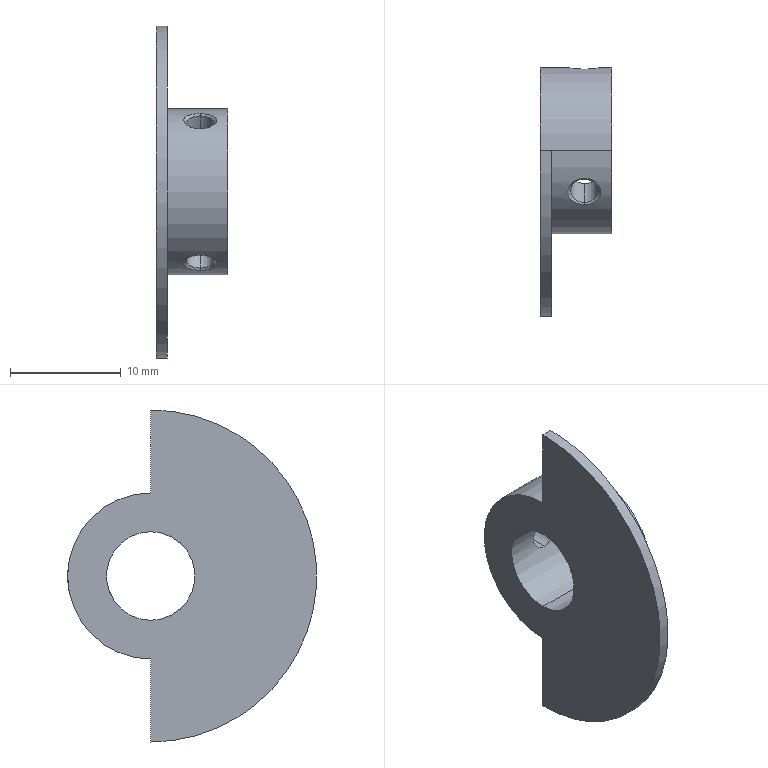Part | SolidWorks | features BaseBody 1 | 1 solid | 22 faces | box 6.5 x 22.5 x 30 mm | volume 1036 mm3 | cylinder 11 | cone 6 | plane 5 | commonest cylinder face diameters 2.459 x6 8 x2 15 x2 30 x1
STEP:
#1=CARTESIAN_POINT('',(4.,7.373,1.373));
#2=VERTEX_POINT('',#1);
#3=CARTESIAN_POINT('',(4.,7.373,-1.373));
#4=VERTEX_POINT('',#3);
#5=CARTESIAN_POINT('',(4.,7.373,1.373));
#6=CARTESIAN_POINT('',(3.812,7.373,1.373));
#7=CARTESIAN_POINT('',(3.623,7.38,1.34));
#8=CARTESIAN_POINT('',(3.27,7.402,1.211));
#9=CARTESIAN_POINT('',(3.105,7.418,1.115));
#10=CARTESIAN_POINT('',(2.821,7.451,0.8664));
#11=CARTESIAN_POINT('',(2.704,7.468,0.7143));
#12=CARTESIAN_POINT('',(2.543,7.493,0.3737));
#13=CARTESIAN_POINT('',(2.5,7.5,0.1847));
#14=CARTESIAN_POINT('',(2.5,7.5,-0.09668));
#15=CARTESIAN_POINT('',(2.511,7.498,-0.1919));
#16=CARTESIAN_POINT('',(2.554,7.491,-0.3755));
#17=CARTESIAN_POINT('',(2.585,7.486,-0.4636));
#18=CARTESIAN_POINT('',(2.666,7.474,-0.6329));
#19=CARTESIAN_POINT('',(2.716,7.466,-0.7143));
#20=CARTESIAN_POINT('',(2.83,7.451,-0.8624));
#21=CARTESIAN_POINT('',(2.894,7.442,-0.9303));
#22=CARTESIAN_POINT('',(3.035,7.426,-1.054));
#23=CARTESIAN_POINT('',(3.113,7.418,-1.109));
#24=CARTESIAN_POINT('',(3.274,7.403,-1.204));
#25=CARTESIAN_POINT('',(3.358,7.396,-1.244));
#26=CARTESIAN_POINT('',(3.624,7.379,-1.341));
#27=CARTESIAN_POINT('',(3.81,7.373,-1.373));
#28=CARTESIAN_POINT('',(4.,7.373,-1.373));
#29=B_SPLINE_CURVE_WITH_KNOTS('',3,(#5,#6,#7,#8,#9,#10,#11,#12,#13,#14,#15,#16,#17,#18,#19,#20,#21,#22,#23,#24,#25,#26,#27,#28),.UNSPECIFIED.,.F.,.F.,(4,2,2,2,2,2,2,2,2,2,2,4),(0.0008214,0.001385,0.001948,0.002512,0.003075,0.003357,0.003639,0.003921,0.004202,0.004484,0.004766,0.005329),.UNSPECIFIED.);
#30=EDGE_CURVE('',#2,#4,#29,.T.);
#31=ORIENTED_EDGE('',*,*,#30,.T.);
#32=CARTESIAN_POINT('',(4.,7.373,-1.373));
#33=CARTESIAN_POINT('',(4.19,7.373,-1.373));
#34=CARTESIAN_POINT('',(4.376,7.379,-1.341));
#35=CARTESIAN_POINT('',(4.731,7.402,-1.211));
#36=CARTESIAN_POINT('',(4.896,7.418,-1.115));
#37=CARTESIAN_POINT('',(5.178,7.451,-0.8673));
#38=CARTESIAN_POINT('',(5.295,7.468,-0.7151));
#39=CARTESIAN_POINT('',(5.416,7.486,-0.461));
#40=CARTESIAN_POINT('',(5.448,7.491,-0.3707));
#41=CARTESIAN_POINT('',(5.489,7.498,-0.1871));
#42=CARTESIAN_POINT('',(5.5,7.5,-0.09388));
#43=CARTESIAN_POINT('',(5.5,7.5,0.19));
#44=CARTESIAN_POINT('',(5.456,7.492,0.3767));
#45=CARTESIAN_POINT('',(5.335,7.474,0.6321));
#46=CARTESIAN_POINT('',(5.286,7.467,0.7115));
#47=CARTESIAN_POINT('',(5.172,7.451,0.8598));
#48=CARTESIAN_POINT('',(5.107,7.442,0.9292));
#49=CARTESIAN_POINT('',(4.895,7.418,1.115));
#50=CARTESIAN_POINT('',(4.73,7.402,1.212));
#51=CARTESIAN_POINT('',(4.377,7.38,1.34));
#52=CARTESIAN_POINT('',(4.188,7.373,1.373));
#53=CARTESIAN_POINT('',(4.,7.373,1.373));
#54=B_SPLINE_CURVE_WITH_KNOTS('',3,(#32,#33,#34,#35,#36,#37,#38,#39,#40,#41,#42,#43,#44,#45,#46,#47,#48,#49,#50,#51,#52,#53),.UNSPECIFIED.,.F.,.F.,(4,2,2,2,2,2,2,2,2,2,4),(0.005329,0.005893,0.006456,0.00702,0.007301,0.007583,0.008146,0.008428,0.00871,0.009273,0.009837),.UNSPECIFIED.);
#55=EDGE_CURVE('',#4,#2,#54,.T.);
#56=ORIENTED_EDGE('',*,*,#55,.T.);
#57=EDGE_LOOP('',(#31,#56));
#58=FACE_BOUND('',#57,.T.);
#59=CARTESIAN_POINT('',(1.,0.,7.5));
#60=VERTEX_POINT('',#59);
#61=CARTESIAN_POINT('',(0.,0.,7.5));
#62=VERTEX_POINT('',#61);
#63=CARTESIAN_POINT('',(1.,0.,7.5));
#64=DIRECTION('',(-1.,0.,0.));
#65=VECTOR('',#64,1000.);
#66=LINE('',#63,#65);
#67=EDGE_CURVE('',#60,#62,#66,.T.);
#68=ORIENTED_EDGE('',*,*,#67,.F.);
#69=CARTESIAN_POINT('',(6.5,0.,7.5));
#70=VERTEX_POINT('',#69);
#71=CARTESIAN_POINT('',(0.,0.,7.5));
#72=DIRECTION('',(1.,0.,0.));
#73=VECTOR('',#72,1000.);
#74=LINE('',#71,#73);
#75=EDGE_CURVE('',#60,#70,#74,.T.);
#76=ORIENTED_EDGE('',*,*,#75,.T.);
#77=CARTESIAN_POINT('',(6.5,0.,-7.5));
#78=VERTEX_POINT('',#77);
#79=CARTESIAN_POINT('',(6.5,0.,0.));
#80=DIRECTION('',(-1.,0.,0.));
#81=DIRECTION('',(0.,0.,-1.));
#82=AXIS2_PLACEMENT_3D('',#79,#80,#81);
#83=CIRCLE('',#82,7.5);
#84=EDGE_CURVE('',#70,#78,#83,.T.);
#85=ORIENTED_EDGE('',*,*,#84,.T.);
#86=CARTESIAN_POINT('',(1.,0.,-7.5));
#87=VERTEX_POINT('',#86);
#88=CARTESIAN_POINT('',(0.,0.,-7.5));
#89=DIRECTION('',(1.,0.,0.));
#90=VECTOR('',#89,1000.);
#91=LINE('',#88,#90);
#92=EDGE_CURVE('',#87,#78,#91,.T.);
#93=ORIENTED_EDGE('',*,*,#92,.F.);
#94=CARTESIAN_POINT('',(0.,0.,-7.5));
#95=VERTEX_POINT('',#94);
#96=CARTESIAN_POINT('',(0.,0.,-7.5));
#97=DIRECTION('',(-1.,0.,0.));
#98=VECTOR('',#97,1000.);
#99=LINE('',#96,#98);
#100=EDGE_CURVE('',#87,#95,#99,.T.);
#101=ORIENTED_EDGE('',*,*,#100,.T.);
#102=CARTESIAN_POINT('',(0.,0.,0.));
#103=DIRECTION('',(1.,0.,0.));
#104=DIRECTION('',(0.,0.,-1.));
#105=AXIS2_PLACEMENT_3D('',#102,#103,#104);
#106=CIRCLE('',#105,7.5);
#107=EDGE_CURVE('',#95,#62,#106,.T.);
#108=ORIENTED_EDGE('',*,*,#107,.T.);
#109=EDGE_LOOP('',(#68,#76,#85,#93,#101,#108));
#110=FACE_OUTER_BOUND('',#109,.T.);
#111=CARTESIAN_POINT('',(0.,0.,0.));
#112=DIRECTION('',(1.,0.,0.));
#113=DIRECTION('',(0.,0.,-1.));
#114=AXIS2_PLACEMENT_3D('',#111,#112,#113);
#115=CYLINDRICAL_SURFACE('',#114,7.5);
#116=ADVANCED_FACE('',(#58,#110),#115,.T.);
#117=CARTESIAN_POINT('',(4.,-2.968,2.682));
#118=VERTEX_POINT('',#117);
#119=CARTESIAN_POINT('',(4.,-0.8384,3.911));
#120=VERTEX_POINT('',#119);
#121=CARTESIAN_POINT('',(4.,-2.968,2.682));
#122=CARTESIAN_POINT('',(3.919,-2.968,2.682));
#123=CARTESIAN_POINT('',(3.837,-2.962,2.688));
#124=CARTESIAN_POINT('',(3.679,-2.94,2.713));
#125=CARTESIAN_POINT('',(3.602,-2.923,2.731));
#126=CARTESIAN_POINT('',(3.379,-2.856,2.801));
#127=CARTESIAN_POINT('',(3.245,-2.791,2.868));
#128=CARTESIAN_POINT('',(3.017,-2.619,3.025));
#129=CARTESIAN_POINT('',(2.926,-2.515,3.114));
#130=CARTESIAN_POINT('',(2.803,-2.275,3.294));
#131=CARTESIAN_POINT('',(2.77,-2.139,3.384));
#132=CARTESIAN_POINT('',(2.771,-1.86,3.545));
#133=CARTESIAN_POINT('',(2.803,-1.714,3.617));
#134=CARTESIAN_POINT('',(2.926,-1.441,3.735));
#135=CARTESIAN_POINT('',(3.017,-1.31,3.781));
#136=CARTESIAN_POINT('',(3.243,-1.089,3.851));
#137=CARTESIAN_POINT('',(3.378,-0.998,3.874));
#138=CARTESIAN_POINT('',(3.677,-0.8717,3.904));
#139=CARTESIAN_POINT('',(3.838,-0.8384,3.911));
#140=CARTESIAN_POINT('',(4.,-0.8384,3.911));
#141=B_SPLINE_CURVE_WITH_KNOTS('',3,(#121,#122,#123,#124,#125,#126,#127,#128,#129,#130,#131,#132,#133,#134,#135,#136,#137,#138,#139,#140),.UNSPECIFIED.,.F.,.F.,(4,2,2,2,2,2,2,2,2,4),(0.0002413,0.0004837,0.0007262,0.001211,0.001696,0.002181,0.002665,0.00315,0.003635,0.00412),.UNSPECIFIED.);
#142=EDGE_CURVE('',#118,#120,#141,.T.);
#143=ORIENTED_EDGE('',*,*,#142,.F.);
#144=CARTESIAN_POINT('',(4.,-0.8384,3.911));
#145=CARTESIAN_POINT('',(4.081,-0.8384,3.911));
#146=CARTESIAN_POINT('',(4.161,-0.8466,3.909));
#147=CARTESIAN_POINT('',(4.319,-0.8789,3.902));
#148=CARTESIAN_POINT('',(4.398,-0.9034,3.897));
#149=CARTESIAN_POINT('',(4.62,-0.9969,3.874));
#150=CARTESIAN_POINT('',(4.756,-1.089,3.851));
#151=CARTESIAN_POINT('',(4.982,-1.309,3.782));
#152=CARTESIAN_POINT('',(5.073,-1.439,3.735));
#153=CARTESIAN_POINT('',(5.166,-1.645,3.647));
#154=CARTESIAN_POINT('',(5.19,-1.717,3.614));
#155=CARTESIAN_POINT('',(5.221,-1.858,3.543));
#156=CARTESIAN_POINT('',(5.229,-1.929,3.505));
#157=CARTESIAN_POINT('',(5.23,-2.141,3.383));
#158=CARTESIAN_POINT('',(5.197,-2.274,3.294));
#159=CARTESIAN_POINT('',(5.073,-2.515,3.114));
#160=CARTESIAN_POINT('',(4.982,-2.62,3.025));
#161=CARTESIAN_POINT('',(4.756,-2.79,2.868));
#162=CARTESIAN_POINT('',(4.62,-2.857,2.801));
#163=CARTESIAN_POINT('',(4.324,-2.945,2.708));
#164=CARTESIAN_POINT('',(4.162,-2.968,2.682));
#165=CARTESIAN_POINT('',(4.,-2.968,2.682));
#166=B_SPLINE_CURVE_WITH_KNOTS('',3,(#144,#145,#146,#147,#148,#149,#150,#151,#152,#153,#154,#155,#156,#157,#158,#159,#160,#161,#162,#163,#164,#165),.UNSPECIFIED.,.F.,.F.,(4,2,2,2,2,2,2,2,2,2,4),(0.00412,0.004362,0.004605,0.00509,0.005575,0.005818,0.00606,0.006545,0.00703,0.007515,0.008),.UNSPECIFIED.);
#167=EDGE_CURVE('',#120,#118,#166,.T.);
#168=ORIENTED_EDGE('',*,*,#167,.F.);
#169=EDGE_LOOP('',(#143,#168));
#170=FACE_BOUND('',#169,.T.);
#171=CARTESIAN_POINT('',(4.,-0.8384,-3.911));
#172=VERTEX_POINT('',#171);
#173=CARTESIAN_POINT('',(4.,-2.968,-2.682));
#174=VERTEX_POINT('',#173);
#175=CARTESIAN_POINT('',(4.,-0.8384,-3.911));
#176=CARTESIAN_POINT('',(3.919,-0.8384,-3.911));
#177=CARTESIAN_POINT('',(3.837,-0.8468,-3.909));
#178=CARTESIAN_POINT('',(3.679,-0.8793,-3.902));
#179=CARTESIAN_POINT('',(3.602,-0.9032,-3.897));
#180=CARTESIAN_POINT('',(3.379,-0.9973,-3.874));
#181=CARTESIAN_POINT('',(3.245,-1.088,-3.851));
#182=CARTESIAN_POINT('',(3.017,-1.311,-3.781));
#183=CARTESIAN_POINT('',(2.926,-1.44,-3.735));
#184=CARTESIAN_POINT('',(2.803,-1.715,-3.617));
#185=CARTESIAN_POINT('',(2.77,-1.861,-3.545));
#186=CARTESIAN_POINT('',(2.771,-2.14,-3.383));
#187=CARTESIAN_POINT('',(2.803,-2.275,-3.293));
#188=CARTESIAN_POINT('',(2.926,-2.514,-3.115));
#189=CARTESIAN_POINT('',(3.017,-2.619,-3.025));
#190=CARTESIAN_POINT('',(3.243,-2.79,-2.869));
#191=CARTESIAN_POINT('',(3.378,-2.856,-2.801));
#192=CARTESIAN_POINT('',(3.677,-2.945,-2.707));
#193=CARTESIAN_POINT('',(3.838,-2.968,-2.682));
#194=CARTESIAN_POINT('',(4.,-2.968,-2.682));
#195=B_SPLINE_CURVE_WITH_KNOTS('',3,(#175,#176,#177,#178,#179,#180,#181,#182,#183,#184,#185,#186,#187,#188,#189,#190,#191,#192,#193,#194),.UNSPECIFIED.,.F.,.F.,(4,2,2,2,2,2,2,2,2,4),(0.0002413,0.0004837,0.0007262,0.001211,0.001696,0.002181,0.002665,0.00315,0.003635,0.00412),.UNSPECIFIED.);
#196=EDGE_CURVE('',#172,#174,#195,.T.);
#197=ORIENTED_EDGE('',*,*,#196,.F.);
#198=CARTESIAN_POINT('',(4.,-2.968,-2.682));
#199=CARTESIAN_POINT('',(4.081,-2.968,-2.682));
#200=CARTESIAN_POINT('',(4.161,-2.962,-2.688));
#201=CARTESIAN_POINT('',(4.319,-2.94,-2.712));
#202=CARTESIAN_POINT('',(4.398,-2.923,-2.731));
#203=CARTESIAN_POINT('',(4.62,-2.857,-2.801));
#204=CARTESIAN_POINT('',(4.756,-2.79,-2.868));
#205=CARTESIAN_POINT('',(4.982,-2.621,-3.024));
#206=CARTESIAN_POINT('',(5.073,-2.515,-3.114));
#207=CARTESIAN_POINT('',(5.166,-2.336,-3.248));
#208=CARTESIAN_POINT('',(5.19,-2.271,-3.294));
#209=CARTESIAN_POINT('',(5.221,-2.139,-3.381));
#210=CARTESIAN_POINT('',(5.229,-2.071,-3.423));
#211=CARTESIAN_POINT('',(5.23,-1.859,-3.545));
#212=CARTESIAN_POINT('',(5.197,-1.715,-3.617));
#213=CARTESIAN_POINT('',(5.073,-1.439,-3.735));
#214=CARTESIAN_POINT('',(4.982,-1.31,-3.781));
#215=CARTESIAN_POINT('',(4.756,-1.089,-3.851));
#216=CARTESIAN_POINT('',(4.62,-0.9971,-3.874));
#217=CARTESIAN_POINT('',(4.324,-0.8723,-3.904));
#218=CARTESIAN_POINT('',(4.162,-0.8384,-3.911));
#219=CARTESIAN_POINT('',(4.,-0.8384,-3.911));
#220=B_SPLINE_CURVE_WITH_KNOTS('',3,(#198,#199,#200,#201,#202,#203,#204,#205,#206,#207,#208,#209,#210,#211,#212,#213,#214,#215,#216,#217,#218,#219),.UNSPECIFIED.,.F.,.F.,(4,2,2,2,2,2,2,2,2,2,4),(0.00412,0.004362,0.004605,0.00509,0.005575,0.005818,0.00606,0.006545,0.00703,0.007515,0.008),.UNSPECIFIED.);
#221=EDGE_CURVE('',#174,#172,#220,.T.);
#222=ORIENTED_EDGE('',*,*,#221,.F.);
#223=EDGE_LOOP('',(#197,#222));
#224=FACE_BOUND('',#223,.T.);
#225=CARTESIAN_POINT('',(0.,0.,-4.));
#226=VERTEX_POINT('',#225);
#227=CARTESIAN_POINT('',(0.,0.,4.));
#228=VERTEX_POINT('',#227);
#229=CARTESIAN_POINT('',(0.,0.,0.));
#230=DIRECTION('',(-1.,0.,0.));
#231=DIRECTION('',(0.,0.,-1.));
#232=AXIS2_PLACEMENT_3D('',#229,#230,#231);
#233=CIRCLE('',#232,4.);
#234=EDGE_CURVE('',#226,#228,#233,.T.);
#235=ORIENTED_EDGE('',*,*,#234,.T.);
#236=CARTESIAN_POINT('',(6.5,0.,4.));
#237=VERTEX_POINT('',#236);
#238=CARTESIAN_POINT('',(6.5,0.,4.));
#239=DIRECTION('',(1.,0.,0.));
#240=VECTOR('',#239,1000.);
#241=LINE('',#238,#240);
#242=EDGE_CURVE('',#228,#237,#241,.T.);
#243=ORIENTED_EDGE('',*,*,#242,.T.);
#244=CARTESIAN_POINT('',(6.5,0.,-4.));
#245=VERTEX_POINT('',#244);
#246=CARTESIAN_POINT('',(6.5,0.,0.));
#247=DIRECTION('',(-1.,0.,0.));
#248=DIRECTION('',(0.,0.,-1.));
#249=AXIS2_PLACEMENT_3D('',#246,#247,#248);
#250=CIRCLE('',#249,4.);
#251=EDGE_CURVE('',#245,#237,#250,.T.);
#252=ORIENTED_EDGE('',*,*,#251,.F.);
#253=CARTESIAN_POINT('',(6.5,0.,-4.));
#254=DIRECTION('',(1.,0.,0.));
#255=VECTOR('',#254,1000.);
#256=LINE('',#253,#255);
#257=EDGE_CURVE('',#226,#245,#256,.T.);
#258=ORIENTED_EDGE('',*,*,#257,.F.);
#259=EDGE_LOOP('',(#235,#243,#252,#258));
#260=FACE_OUTER_BOUND('',#259,.T.);
#261=CARTESIAN_POINT('',(6.5,0.,0.));
#262=DIRECTION('',(1.,0.,0.));
#263=DIRECTION('',(0.,0.,-1.));
#264=AXIS2_PLACEMENT_3D('',#261,#262,#263);
#265=CYLINDRICAL_SURFACE('',#264,4.);
#266=ADVANCED_FACE('',(#170,#224,#260),#265,.F.);
#267=CARTESIAN_POINT('',(4.,-4.68,-5.646));
#268=VERTEX_POINT('',#267);
#269=CARTESIAN_POINT('',(4.,-2.55,-6.876));
#270=VERTEX_POINT('',#269);
#271=CARTESIAN_POINT('',(4.,-3.615,-6.261));
#272=DIRECTION('',(0.,-0.5,-0.866));
#273=DIRECTION('',(0.,0.866,-0.5));
#274=AXIS2_PLACEMENT_3D('',#271,#272,#273);
#275=CIRCLE('',#274,1.229);
#276=EDGE_CURVE('',#268,#270,#275,.T.);
#277=ORIENTED_EDGE('',*,*,#276,.F.);
#278=CARTESIAN_POINT('',(4.,-4.876,-5.699));
#279=VERTEX_POINT('',#278);
#280=CARTESIAN_POINT('',(4.,-5.053,-5.746));
#281=DIRECTION('',(0.,-0.9659,-0.2588));
#282=VECTOR('',#281,1000.);
#283=LINE('',#280,#282);
#284=EDGE_CURVE('',#268,#279,#283,.T.);
#285=ORIENTED_EDGE('',*,*,#284,.T.);
#286=CARTESIAN_POINT('',(4.,-2.497,-7.072));
#287=VERTEX_POINT('',#286);
#288=CARTESIAN_POINT('',(4.,-2.497,-7.072));
#289=CARTESIAN_POINT('',(3.812,-2.497,-7.072));
#290=CARTESIAN_POINT('',(3.623,-2.529,-7.061));
#291=CARTESIAN_POINT('',(3.27,-2.652,-7.016));
#292=CARTESIAN_POINT('',(3.105,-2.743,-6.982));
#293=CARTESIAN_POINT('',(2.821,-2.975,-6.886));
#294=CARTESIAN_POINT('',(2.704,-3.115,-6.825));
#295=CARTESIAN_POINT('',(2.543,-3.423,-6.676));
#296=CARTESIAN_POINT('',(2.5,-3.59,-6.588));
#297=CARTESIAN_POINT('',(2.5,-3.834,-6.447));
#298=CARTESIAN_POINT('',(2.511,-3.915,-6.398));
#299=CARTESIAN_POINT('',(2.554,-4.071,-6.3));
#300=CARTESIAN_POINT('',(2.585,-4.145,-6.251));
#301=CARTESIAN_POINT('',(2.666,-4.285,-6.156));
#302=CARTESIAN_POINT('',(2.716,-4.352,-6.109));
#303=CARTESIAN_POINT('',(2.83,-4.472,-6.021));
#304=CARTESIAN_POINT('',(2.894,-4.527,-5.98));
#305=CARTESIAN_POINT('',(3.035,-4.626,-5.904));
#306=CARTESIAN_POINT('',(3.113,-4.67,-5.869));
#307=CARTESIAN_POINT('',(3.274,-4.744,-5.809));
#308=CARTESIAN_POINT('',(3.358,-4.775,-5.784));
#309=CARTESIAN_POINT('',(3.624,-4.851,-5.721));
#310=CARTESIAN_POINT('',(3.811,-4.876,-5.699));
#311=CARTESIAN_POINT('',(4.,-4.876,-5.699));
#312=B_SPLINE_CURVE_WITH_KNOTS('',3,(#288,#289,#290,#291,#292,#293,#294,#295,#296,#297,#298,#299,#300,#301,#302,#303,#304,#305,#306,#307,#308,#309,#310,#311),.UNSPECIFIED.,.F.,.F.,(4,2,2,2,2,2,2,2,2,2,2,4),(0.001763,0.002329,0.002895,0.003461,0.004027,0.00431,0.004593,0.004876,0.005159,0.005442,0.005725,0.006291),.UNSPECIFIED.);
#313=EDGE_CURVE('',#287,#279,#312,.T.);
#314=ORIENTED_EDGE('',*,*,#313,.F.);
#315=CARTESIAN_POINT('',(4.,-2.45,-7.249));
#316=DIRECTION('',(0.,0.2588,-0.9659));
#317=VECTOR('',#316,1000.);
#318=LINE('',#315,#317);
#319=EDGE_CURVE('',#270,#287,#318,.T.);
#320=ORIENTED_EDGE('',*,*,#319,.F.);
#321=EDGE_LOOP('',(#277,#285,#314,#320));
#322=FACE_OUTER_BOUND('',#321,.T.);
#323=CARTESIAN_POINT('',(4.,-3.751,-6.498));
#324=DIRECTION('',(0.,-0.5,-0.866));
#325=DIRECTION('',(0.,0.866,-0.5));
#326=AXIS2_PLACEMENT_3D('',#323,#324,#325);
#327=CONICAL_SURFACE('',#326,1.503,0.7854);
#328=ADVANCED_FACE('',(#322),#327,.F.);
#329=CARTESIAN_POINT('',(4.,7.229,-1.23));
#330=VERTEX_POINT('',#329);
#331=CARTESIAN_POINT('',(4.,7.229,1.23));
#332=VERTEX_POINT('',#331);
#333=CARTESIAN_POINT('',(4.,7.229,0.));
#334=DIRECTION('',(0.,1.,0.));
#335=DIRECTION('',(0.,0.,1.));
#336=AXIS2_PLACEMENT_3D('',#333,#334,#335);
#337=CIRCLE('',#336,1.23);
#338=EDGE_CURVE('',#330,#332,#337,.T.);
#339=ORIENTED_EDGE('',*,*,#338,.F.);
#340=CARTESIAN_POINT('',(4.,7.502,-1.502));
#341=DIRECTION('',(0.,0.7071,-0.7071));
#342=VECTOR('',#341,1000.);
#343=LINE('',#340,#342);
#344=EDGE_CURVE('',#330,#4,#343,.T.);
#345=ORIENTED_EDGE('',*,*,#344,.T.);
#346=ORIENTED_EDGE('',*,*,#30,.F.);
#347=CARTESIAN_POINT('',(4.,7.502,1.502));
#348=DIRECTION('',(0.,0.7071,0.7071));
#349=VECTOR('',#348,1000.);
#350=LINE('',#347,#349);
#351=EDGE_CURVE('',#332,#2,#350,.T.);
#352=ORIENTED_EDGE('',*,*,#351,.F.);
#353=EDGE_LOOP('',(#339,#345,#346,#352));
#354=FACE_OUTER_BOUND('',#353,.T.);
#355=CARTESIAN_POINT('',(4.,7.502,0.));
#356=DIRECTION('',(0.,1.,0.));
#357=DIRECTION('',(0.,0.,1.));
#358=AXIS2_PLACEMENT_3D('',#355,#356,#357);
#359=CONICAL_SURFACE('',#358,1.502,0.7854);
#360=ADVANCED_FACE('',(#354),#359,.F.);
#361=CARTESIAN_POINT('',(4.,-2.55,6.876));
#362=VERTEX_POINT('',#361);
#363=CARTESIAN_POINT('',(4.,-4.68,5.646));
#364=VERTEX_POINT('',#363);
#365=CARTESIAN_POINT('',(4.,-3.615,6.261));
#366=DIRECTION('',(0.,-0.5,0.866));
#367=DIRECTION('',(0.,-0.866,-0.5));
#368=AXIS2_PLACEMENT_3D('',#365,#366,#367);
#369=CIRCLE('',#368,1.229);
#370=EDGE_CURVE('',#362,#364,#369,.T.);
#371=ORIENTED_EDGE('',*,*,#370,.F.);
#372=CARTESIAN_POINT('',(4.,-2.497,7.072));
#373=VERTEX_POINT('',#372);
#374=CARTESIAN_POINT('',(4.,-2.45,7.249));
#375=DIRECTION('',(0.,0.2588,0.9659));
#376=VECTOR('',#375,1000.);
#377=LINE('',#374,#376);
#378=EDGE_CURVE('',#362,#373,#377,.T.);
#379=ORIENTED_EDGE('',*,*,#378,.T.);
#380=CARTESIAN_POINT('',(4.,-4.876,5.699));
#381=VERTEX_POINT('',#380);
#382=CARTESIAN_POINT('',(4.,-4.876,5.699));
#383=CARTESIAN_POINT('',(3.812,-4.876,5.699));
#384=CARTESIAN_POINT('',(3.623,-4.85,5.721));
#385=CARTESIAN_POINT('',(3.27,-4.75,5.804));
#386=CARTESIAN_POINT('',(3.104,-4.674,5.867));
#387=CARTESIAN_POINT('',(2.822,-4.476,6.019));
#388=CARTESIAN_POINT('',(2.705,-4.354,6.109));
#389=CARTESIAN_POINT('',(2.583,-4.14,6.254));
#390=CARTESIAN_POINT('',(2.552,-4.066,6.303));
#391=CARTESIAN_POINT('',(2.51,-3.91,6.401));
#392=CARTESIAN_POINT('',(2.5,-3.829,6.45));
#393=CARTESIAN_POINT('',(2.5,-3.585,6.591));
#394=CARTESIAN_POINT('',(2.545,-3.417,6.679));
#395=CARTESIAN_POINT('',(2.666,-3.189,6.789));
#396=CARTESIAN_POINT('',(2.716,-3.115,6.823));
#397=CARTESIAN_POINT('',(2.83,-2.978,6.884));
#398=CARTESIAN_POINT('',(2.894,-2.915,6.911));
#399=CARTESIAN_POINT('',(3.035,-2.8,6.958));
#400=CARTESIAN_POINT('',(3.112,-2.748,6.979));
#401=CARTESIAN_POINT('',(3.274,-2.659,7.013));
#402=CARTESIAN_POINT('',(3.359,-2.621,7.027));
#403=CARTESIAN_POINT('',(3.535,-2.56,7.05));
#404=CARTESIAN_POINT('',(3.627,-2.536,7.058));
#405=CARTESIAN_POINT('',(3.813,-2.505,7.069));
#406=CARTESIAN_POINT('',(3.906,-2.497,7.072));
#407=CARTESIAN_POINT('',(4.,-2.497,7.072));
#408=B_SPLINE_CURVE_WITH_KNOTS('',3,(#382,#383,#384,#385,#386,#387,#388,#389,#390,#391,#392,#393,#394,#395,#396,#397,#398,#399,#400,#401,#402,#403,#404,#405,#406,#407),.UNSPECIFIED.,.F.,.F.,(4,2,2,2,2,2,2,2,2,2,2,2,4),(0.002987,0.003555,0.004124,0.004692,0.004976,0.005261,0.005829,0.006113,0.006398,0.006682,0.006966,0.00725,0.007535),.UNSPECIFIED.);
#409=EDGE_CURVE('',#381,#373,#408,.T.);
#410=ORIENTED_EDGE('',*,*,#409,.F.);
#411=CARTESIAN_POINT('',(4.,-5.053,5.746));
#412=DIRECTION('',(0.,-0.9659,0.2588));
#413=VECTOR('',#412,1000.);
#414=LINE('',#411,#413);
#415=EDGE_CURVE('',#364,#381,#414,.T.);
#416=ORIENTED_EDGE('',*,*,#415,.F.);
#417=EDGE_LOOP('',(#371,#379,#410,#416));
#418=FACE_OUTER_BOUND('',#417,.T.);
#419=CARTESIAN_POINT('',(4.,-3.751,6.498));
#420=DIRECTION('',(0.,-0.5,0.866));
#421=DIRECTION('',(0.,-0.866,-0.5));
#422=AXIS2_PLACEMENT_3D('',#419,#420,#421);
#423=CONICAL_SURFACE('',#422,1.503,0.7854);
#424=ADVANCED_FACE('',(#418),#423,.F.);
#425=ORIENTED_EDGE('',*,*,#196,.T.);
#426=CARTESIAN_POINT('',(4.,-2.565,-1.983));
#427=DIRECTION('',(0.,-0.5,-0.866));
#428=VECTOR('',#427,1000.);
#429=LINE('',#426,#428);
#430=EDGE_CURVE('',#174,#268,#429,.T.);
#431=ORIENTED_EDGE('',*,*,#430,.T.);
#432=ORIENTED_EDGE('',*,*,#276,.T.);
#433=CARTESIAN_POINT('',(4.,-0.4352,-3.213));
#434=DIRECTION('',(0.,-0.5,-0.866));
#435=VECTOR('',#434,1000.);
#436=LINE('',#433,#435);
#437=EDGE_CURVE('',#172,#270,#436,.T.);
#438=ORIENTED_EDGE('',*,*,#437,.F.);
#439=EDGE_LOOP('',(#425,#431,#432,#438));
#440=FACE_OUTER_BOUND('',#439,.T.);
#441=CARTESIAN_POINT('',(4.,-1.5,-2.598));
#442=DIRECTION('',(0.,-0.5,-0.866));
#443=DIRECTION('',(0.,0.866,-0.5));
#444=AXIS2_PLACEMENT_3D('',#441,#442,#443);
#445=CYLINDRICAL_SURFACE('',#444,1.23);
#446=ADVANCED_FACE('',(#440),#445,.F.);
#447=ORIENTED_EDGE('',*,*,#142,.T.);
#448=CARTESIAN_POINT('',(4.,-0.4352,3.213));
#449=DIRECTION('',(0.,-0.5,0.866));
#450=VECTOR('',#449,1000.);
#451=LINE('',#448,#450);
#452=EDGE_CURVE('',#120,#362,#451,.T.);
#453=ORIENTED_EDGE('',*,*,#452,.T.);
#454=ORIENTED_EDGE('',*,*,#370,.T.);
#455=CARTESIAN_POINT('',(4.,-2.565,1.983));
#456=DIRECTION('',(0.,-0.5,0.866));
#457=VECTOR('',#456,1000.);
#458=LINE('',#455,#457);
#459=EDGE_CURVE('',#118,#364,#458,.T.);
#460=ORIENTED_EDGE('',*,*,#459,.F.);
#461=EDGE_LOOP('',(#447,#453,#454,#460));
#462=FACE_OUTER_BOUND('',#461,.T.);
#463=CARTESIAN_POINT('',(4.,-1.5,2.598));
#464=DIRECTION('',(0.,-0.5,0.866));
#465=DIRECTION('',(0.,-0.866,-0.5));
#466=AXIS2_PLACEMENT_3D('',#463,#464,#465);
#467=CYLINDRICAL_SURFACE('',#466,1.23);
#468=ADVANCED_FACE('',(#462),#467,.F.);
#469=CARTESIAN_POINT('',(4.,3.806,1.23));
#470=VERTEX_POINT('',#469);
#471=CARTESIAN_POINT('',(4.,3.806,-1.23));
#472=VERTEX_POINT('',#471);
#473=CARTESIAN_POINT('',(4.,3.806,1.23));
#474=CARTESIAN_POINT('',(3.919,3.806,1.23));
#475=CARTESIAN_POINT('',(3.837,3.809,1.221));
#476=CARTESIAN_POINT('',(3.679,3.819,1.19));
#477=CARTESIAN_POINT('',(3.602,3.826,1.166));
#478=CARTESIAN_POINT('',(3.379,3.854,1.073));
#479=CARTESIAN_POINT('',(3.245,3.879,0.9834));
#480=CARTESIAN_POINT('',(3.017,3.93,0.7555));
#481=CARTESIAN_POINT('',(2.926,3.954,0.6205));
#482=CARTESIAN_POINT('',(2.803,3.99,0.3233));
#483=CARTESIAN_POINT('',(2.77,4.,0.1609));
#484=CARTESIAN_POINT('',(2.771,4.,-0.1613));
#485=CARTESIAN_POINT('',(2.803,3.99,-0.324));
#486=CARTESIAN_POINT('',(2.926,3.955,-0.6197));
#487=CARTESIAN_POINT('',(3.017,3.93,-0.7558));
#488=CARTESIAN_POINT('',(3.243,3.879,-0.9819));
#489=CARTESIAN_POINT('',(3.378,3.854,-1.073));
#490=CARTESIAN_POINT('',(3.677,3.817,-1.197));
#491=CARTESIAN_POINT('',(3.838,3.806,-1.23));
#492=CARTESIAN_POINT('',(4.,3.806,-1.23));
#493=B_SPLINE_CURVE_WITH_KNOTS('',3,(#473,#474,#475,#476,#477,#478,#479,#480,#481,#482,#483,#484,#485,#486,#487,#488,#489,#490,#491,#492),.UNSPECIFIED.,.F.,.F.,(4,2,2,2,2,2,2,2,2,4),(0.0002413,0.0004837,0.0007262,0.001211,0.001696,0.002181,0.002665,0.00315,0.003635,0.00412),.UNSPECIFIED.);
#494=EDGE_CURVE('',#470,#472,#493,.T.);
#495=ORIENTED_EDGE('',*,*,#494,.T.);
#496=CARTESIAN_POINT('',(4.,3.,-1.23));
#497=DIRECTION('',(0.,1.,0.));
#498=VECTOR('',#497,1000.);
#499=LINE('',#496,#498);
#500=EDGE_CURVE('',#472,#330,#499,.T.);
#501=ORIENTED_EDGE('',*,*,#500,.T.);
#502=ORIENTED_EDGE('',*,*,#338,.T.);
#503=CARTESIAN_POINT('',(4.,3.,1.23));
#504=DIRECTION('',(0.,1.,0.));
#505=VECTOR('',#504,1000.);
#506=LINE('',#503,#505);
#507=EDGE_CURVE('',#470,#332,#506,.T.);
#508=ORIENTED_EDGE('',*,*,#507,.F.);
#509=EDGE_LOOP('',(#495,#501,#502,#508));
#510=FACE_OUTER_BOUND('',#509,.T.);
#511=CARTESIAN_POINT('',(4.,3.,0.));
#512=DIRECTION('',(0.,1.,0.));
#513=DIRECTION('',(0.,0.,1.));
#514=AXIS2_PLACEMENT_3D('',#511,#512,#513);
#515=CYLINDRICAL_SURFACE('',#514,1.23);
#516=ADVANCED_FACE('',(#510),#515,.F.);
#517=ORIENTED_EDGE('',*,*,#107,.F.);
#518=CARTESIAN_POINT('',(0.,0.,-15.));
#519=VERTEX_POINT('',#518);
#520=CARTESIAN_POINT('',(0.,0.,0.));
#521=DIRECTION('',(0.,0.,1.));
#522=VECTOR('',#521,1000.);
#523=LINE('',#520,#522);
#524=EDGE_CURVE('',#519,#95,#523,.T.);
#525=ORIENTED_EDGE('',*,*,#524,.F.);
#526=CARTESIAN_POINT('',(0.,0.,15.));
#527=VERTEX_POINT('',#526);
#528=CARTESIAN_POINT('',(0.,0.,0.));
#529=DIRECTION('',(1.,0.,0.));
#530=DIRECTION('',(0.,0.,-1.));
#531=AXIS2_PLACEMENT_3D('',#528,#529,#530);
#532=CIRCLE('',#531,15.);
#533=EDGE_CURVE('',#527,#519,#532,.T.);
#534=ORIENTED_EDGE('',*,*,#533,.F.);
#535=CARTESIAN_POINT('',(0.,0.,0.));
#536=DIRECTION('',(0.,0.,1.));
#537=VECTOR('',#536,1000.);
#538=LINE('',#535,#537);
#539=EDGE_CURVE('',#62,#527,#538,.T.);
#540=ORIENTED_EDGE('',*,*,#539,.F.);
#541=EDGE_LOOP('',(#517,#525,#534,#540));
#542=FACE_OUTER_BOUND('',#541,.T.);
#543=ORIENTED_EDGE('',*,*,#234,.F.);
#544=CARTESIAN_POINT('',(0.,0.,0.));
#545=DIRECTION('',(-1.,0.,0.));
#546=DIRECTION('',(0.,0.,-1.));
#547=AXIS2_PLACEMENT_3D('',#544,#545,#546);
#548=CIRCLE('',#547,4.);
#549=EDGE_CURVE('',#228,#226,#548,.T.);
#550=ORIENTED_EDGE('',*,*,#549,.F.);
#551=EDGE_LOOP('',(#543,#550));
#552=FACE_BOUND('',#551,.T.);
#553=CARTESIAN_POINT('',(0.,-15.,0.));
#554=DIRECTION('',(1.,0.,0.));
#555=DIRECTION('',(0.,0.,-1.));
#556=AXIS2_PLACEMENT_3D('',#553,#554,#555);
#557=PLANE('',#556);
#558=ADVANCED_FACE('',(#542,#552),#557,.F.);
#559=CARTESIAN_POINT('',(1.,0.,15.));
#560=VERTEX_POINT('',#559);
#561=CARTESIAN_POINT('',(1.,0.,15.));
#562=DIRECTION('',(0.,0.,-1.));
#563=VECTOR('',#562,1000.);
#564=LINE('',#561,#563);
#565=EDGE_CURVE('',#560,#60,#564,.T.);
#566=ORIENTED_EDGE('',*,*,#565,.T.);
#567=ORIENTED_EDGE('',*,*,#67,.T.);
#568=ORIENTED_EDGE('',*,*,#539,.T.);
#569=CARTESIAN_POINT('',(1.,0.,15.));
#570=DIRECTION('',(1.,0.,0.));
#571=VECTOR('',#570,1000.);
#572=LINE('',#569,#571);
#573=EDGE_CURVE('',#527,#560,#572,.T.);
#574=ORIENTED_EDGE('',*,*,#573,.T.);
#575=EDGE_LOOP('',(#566,#567,#568,#574));
#576=FACE_OUTER_BOUND('',#575,.T.);
#577=CARTESIAN_POINT('',(1.,0.,15.));
#578=DIRECTION('',(0.,1.,0.));
#579=DIRECTION('',(0.,0.,1.));
#580=AXIS2_PLACEMENT_3D('',#577,#578,#579);
#581=PLANE('',#580);
#582=ADVANCED_FACE('',(#576),#581,.T.);
#583=ORIENTED_EDGE('',*,*,#75,.F.);
#584=CARTESIAN_POINT('',(1.,0.,0.));
#585=DIRECTION('',(1.,0.,0.));
#586=DIRECTION('',(0.,0.,-1.));
#587=AXIS2_PLACEMENT_3D('',#584,#585,#586);
#588=CIRCLE('',#587,7.5);
#589=EDGE_CURVE('',#60,#87,#588,.T.);
#590=ORIENTED_EDGE('',*,*,#589,.T.);
#591=ORIENTED_EDGE('',*,*,#92,.T.);
#592=CARTESIAN_POINT('',(6.5,0.,0.));
#593=DIRECTION('',(-1.,0.,0.));
#594=DIRECTION('',(0.,0.,-1.));
#595=AXIS2_PLACEMENT_3D('',#592,#593,#594);
#596=CIRCLE('',#595,7.5);
#597=EDGE_CURVE('',#78,#70,#596,.T.);
#598=ORIENTED_EDGE('',*,*,#597,.T.);
#599=EDGE_LOOP('',(#583,#590,#591,#598));
#600=FACE_OUTER_BOUND('',#599,.T.);
#601=ORIENTED_EDGE('',*,*,#313,.T.);
#602=CARTESIAN_POINT('',(4.,-4.876,-5.699));
#603=CARTESIAN_POINT('',(4.189,-4.876,-5.699));
#604=CARTESIAN_POINT('',(4.376,-4.851,-5.72));
#605=CARTESIAN_POINT('',(4.731,-4.75,-5.805));
#606=CARTESIAN_POINT('',(4.895,-4.675,-5.866));
#607=CARTESIAN_POINT('',(5.178,-4.477,-6.019));
#608=CARTESIAN_POINT('',(5.295,-4.353,-6.11));
#609=CARTESIAN_POINT('',(5.416,-4.143,-6.253));
#610=CARTESIAN_POINT('',(5.448,-4.067,-6.302));
#611=CARTESIAN_POINT('',(5.489,-3.911,-6.4));
#612=CARTESIAN_POINT('',(5.5,-3.832,-6.448));
#613=CARTESIAN_POINT('',(5.5,-3.586,-6.59));
#614=CARTESIAN_POINT('',(5.457,-3.42,-6.677));
#615=CARTESIAN_POINT('',(5.294,-3.112,-6.826));
#616=CARTESIAN_POINT('',(5.176,-2.972,-6.887));
#617=CARTESIAN_POINT('',(4.895,-2.743,-6.981));
#618=CARTESIAN_POINT('',(4.729,-2.651,-7.016));
#619=CARTESIAN_POINT('',(4.377,-2.529,-7.061));
#620=CARTESIAN_POINT('',(4.188,-2.497,-7.072));
#621=CARTESIAN_POINT('',(4.,-2.497,-7.072));
#622=B_SPLINE_CURVE_WITH_KNOTS('',3,(#602,#603,#604,#605,#606,#607,#608,#609,#610,#611,#612,#613,#614,#615,#616,#617,#618,#619,#620,#621),.UNSPECIFIED.,.F.,.F.,(4,2,2,2,2,2,2,2,2,4),(0.006291,0.006857,0.007423,0.007988,0.008271,0.008554,0.00912,0.009686,0.01025,0.01082),.UNSPECIFIED.);
#623=EDGE_CURVE('',#279,#287,#622,.T.);
#624=ORIENTED_EDGE('',*,*,#623,.T.);
#625=EDGE_LOOP('',(#601,#624));
#626=FACE_BOUND('',#625,.T.);
#627=ORIENTED_EDGE('',*,*,#409,.T.);
#628=CARTESIAN_POINT('',(4.,-2.497,7.072));
#629=CARTESIAN_POINT('',(4.094,-2.497,7.072));
#630=CARTESIAN_POINT('',(4.189,-2.505,7.069));
#631=CARTESIAN_POINT('',(4.374,-2.536,7.058));
#632=CARTESIAN_POINT('',(4.465,-2.56,7.05));
#633=CARTESIAN_POINT('',(4.73,-2.652,7.016));
#634=CARTESIAN_POINT('',(4.894,-2.742,6.982));
#635=CARTESIAN_POINT('',(5.107,-2.917,6.91));
#636=CARTESIAN_POINT('',(5.171,-2.98,6.883));
#637=CARTESIAN_POINT('',(5.285,-3.117,6.822));
#638=CARTESIAN_POINT('',(5.335,-3.191,6.788));
#639=CARTESIAN_POINT('',(5.457,-3.422,6.676));
#640=CARTESIAN_POINT('',(5.5,-3.587,6.589));
#641=CARTESIAN_POINT('',(5.5,-3.835,6.446));
#642=CARTESIAN_POINT('',(5.489,-3.914,6.398));
#643=CARTESIAN_POINT('',(5.447,-4.069,6.301));
#644=CARTESIAN_POINT('',(5.415,-4.145,6.251));
#645=CARTESIAN_POINT('',(5.334,-4.285,6.156));
#646=CARTESIAN_POINT('',(5.285,-4.351,6.11));
#647=CARTESIAN_POINT('',(5.171,-4.471,6.022));
#648=CARTESIAN_POINT('',(5.105,-4.527,5.98));
#649=CARTESIAN_POINT('',(4.894,-4.675,5.866));
#650=CARTESIAN_POINT('',(4.729,-4.75,5.804));
#651=CARTESIAN_POINT('',(4.377,-4.85,5.721));
#652=CARTESIAN_POINT('',(4.187,-4.876,5.699));
#653=CARTESIAN_POINT('',(4.,-4.876,5.699));
#654=B_SPLINE_CURVE_WITH_KNOTS('',3,(#628,#629,#630,#631,#632,#633,#634,#635,#636,#637,#638,#639,#640,#641,#642,#643,#644,#645,#646,#647,#648,#649,#650,#651,#652,#653),.UNSPECIFIED.,.F.,.F.,(4,2,2,2,2,2,2,2,2,2,2,2,4),(0.007535,0.007819,0.008103,0.008671,0.008955,0.009239,0.009807,0.01009,0.01037,0.01066,0.01094,0.01151,0.01208),.UNSPECIFIED.);
#655=EDGE_CURVE('',#373,#381,#654,.T.);
#656=ORIENTED_EDGE('',*,*,#655,.T.);
#657=EDGE_LOOP('',(#627,#656));
#658=FACE_BOUND('',#657,.T.);
#659=CARTESIAN_POINT('',(0.,0.,0.));
#660=DIRECTION('',(1.,0.,0.));
#661=DIRECTION('',(0.,0.,-1.));
#662=AXIS2_PLACEMENT_3D('',#659,#660,#661);
#663=CYLINDRICAL_SURFACE('',#662,7.5);
#664=ADVANCED_FACE('',(#600,#626,#658),#663,.T.);
#665=CARTESIAN_POINT('',(1.,0.,-15.));
#666=VERTEX_POINT('',#665);
#667=CARTESIAN_POINT('',(1.,0.,-7.5));
#668=DIRECTION('',(0.,0.,-1.));
#669=VECTOR('',#668,1000.);
#670=LINE('',#667,#669);
#671=EDGE_CURVE('',#87,#666,#670,.T.);
#672=ORIENTED_EDGE('',*,*,#671,.T.);
#673=CARTESIAN_POINT('',(1.,0.,-15.));
#674=DIRECTION('',(-1.,0.,0.));
#675=VECTOR('',#674,1000.);
#676=LINE('',#673,#675);
#677=EDGE_CURVE('',#666,#519,#676,.T.);
#678=ORIENTED_EDGE('',*,*,#677,.T.);
#679=ORIENTED_EDGE('',*,*,#524,.T.);
#680=ORIENTED_EDGE('',*,*,#100,.F.);
#681=EDGE_LOOP('',(#672,#678,#679,#680));
#682=FACE_OUTER_BOUND('',#681,.T.);
#683=CARTESIAN_POINT('',(1.,0.,-7.5));
#684=DIRECTION('',(0.,1.,0.));
#685=DIRECTION('',(0.,0.,1.));
#686=AXIS2_PLACEMENT_3D('',#683,#684,#685);
#687=PLANE('',#686);
#688=ADVANCED_FACE('',(#682),#687,.T.);
#689=ORIENTED_EDGE('',*,*,#573,.F.);
#690=ORIENTED_EDGE('',*,*,#533,.T.);
#691=ORIENTED_EDGE('',*,*,#677,.F.);
#692=CARTESIAN_POINT('',(1.,0.,0.));
#693=DIRECTION('',(-1.,0.,0.));
#694=DIRECTION('',(0.,0.,-1.));
#695=AXIS2_PLACEMENT_3D('',#692,#693,#694);
#696=CIRCLE('',#695,15.);
#697=EDGE_CURVE('',#666,#560,#696,.T.);
#698=ORIENTED_EDGE('',*,*,#697,.T.);
#699=EDGE_LOOP('',(#689,#690,#691,#698));
#700=FACE_OUTER_BOUND('',#699,.T.);
#701=CARTESIAN_POINT('',(0.,0.,0.));
#702=DIRECTION('',(1.,0.,0.));
#703=DIRECTION('',(0.,0.,-1.));
#704=AXIS2_PLACEMENT_3D('',#701,#702,#703);
#705=CYLINDRICAL_SURFACE('',#704,15.);
#706=ADVANCED_FACE('',(#700),#705,.T.);
#707=ORIENTED_EDGE('',*,*,#242,.F.);
#708=ORIENTED_EDGE('',*,*,#549,.T.);
#709=ORIENTED_EDGE('',*,*,#257,.T.);
#710=CARTESIAN_POINT('',(6.5,0.,0.));
#711=DIRECTION('',(-1.,0.,0.));
#712=DIRECTION('',(0.,0.,-1.));
#713=AXIS2_PLACEMENT_3D('',#710,#711,#712);
#714=CIRCLE('',#713,4.);
#715=EDGE_CURVE('',#237,#245,#714,.T.);
#716=ORIENTED_EDGE('',*,*,#715,.F.);
#717=EDGE_LOOP('',(#707,#708,#709,#716));
#718=FACE_OUTER_BOUND('',#717,.T.);
#719=ORIENTED_EDGE('',*,*,#494,.F.);
#720=CARTESIAN_POINT('',(4.,3.806,-1.23));
#721=CARTESIAN_POINT('',(4.081,3.806,-1.229));
#722=CARTESIAN_POINT('',(4.161,3.809,-1.222));
#723=CARTESIAN_POINT('',(4.319,3.819,-1.19));
#724=CARTESIAN_POINT('',(4.398,3.826,-1.166));
#725=CARTESIAN_POINT('',(4.62,3.854,-1.074));
#726=CARTESIAN_POINT('',(4.756,3.879,-0.9825));
#727=CARTESIAN_POINT('',(4.982,3.929,-0.7573));
#728=CARTESIAN_POINT('',(5.073,3.954,-0.6212));
#729=CARTESIAN_POINT('',(5.166,3.981,-0.3987));
#730=CARTESIAN_POINT('',(5.19,3.988,-0.3201));
#731=CARTESIAN_POINT('',(5.221,3.998,-0.162));
#732=CARTESIAN_POINT('',(5.229,4.,-0.08179));
#733=CARTESIAN_POINT('',(5.23,4.,0.1625));
#734=CARTESIAN_POINT('',(5.197,3.99,0.3228));
#735=CARTESIAN_POINT('',(5.073,3.954,0.6216));
#736=CARTESIAN_POINT('',(4.982,3.93,0.7564));
#737=CARTESIAN_POINT('',(4.756,3.879,0.9825));
#738=CARTESIAN_POINT('',(4.62,3.854,1.074));
#739=CARTESIAN_POINT('',(4.324,3.817,1.197));
#740=CARTESIAN_POINT('',(4.162,3.806,1.229));
#741=CARTESIAN_POINT('',(4.,3.806,1.23));
#742=B_SPLINE_CURVE_WITH_KNOTS('',3,(#720,#721,#722,#723,#724,#725,#726,#727,#728,#729,#730,#731,#732,#733,#734,#735,#736,#737,#738,#739,#740,#741),.UNSPECIFIED.,.F.,.F.,(4,2,2,2,2,2,2,2,2,2,4),(0.00412,0.004362,0.004605,0.00509,0.005575,0.005818,0.00606,0.006545,0.00703,0.007515,0.008),.UNSPECIFIED.);
#743=EDGE_CURVE('',#472,#470,#742,.T.);
#744=ORIENTED_EDGE('',*,*,#743,.F.);
#745=EDGE_LOOP('',(#719,#744));
#746=FACE_BOUND('',#745,.T.);
#747=CARTESIAN_POINT('',(6.5,0.,0.));
#748=DIRECTION('',(1.,0.,0.));
#749=DIRECTION('',(0.,0.,-1.));
#750=AXIS2_PLACEMENT_3D('',#747,#748,#749);
#751=CYLINDRICAL_SURFACE('',#750,4.);
#752=ADVANCED_FACE('',(#718,#746),#751,.F.);
#753=ORIENTED_EDGE('',*,*,#589,.F.);
#754=ORIENTED_EDGE('',*,*,#565,.F.);
#755=ORIENTED_EDGE('',*,*,#697,.F.);
#756=ORIENTED_EDGE('',*,*,#671,.F.);
#757=EDGE_LOOP('',(#753,#754,#755,#756));
#758=FACE_OUTER_BOUND('',#757,.T.);
#759=CARTESIAN_POINT('',(1.,-7.5,0.));
#760=DIRECTION('',(-1.,0.,0.));
#761=DIRECTION('',(0.,0.,1.));
#762=AXIS2_PLACEMENT_3D('',#759,#760,#761);
#763=PLANE('',#762);
#764=ADVANCED_FACE('',(#758),#763,.F.);
#765=ORIENTED_EDGE('',*,*,#284,.F.);
#766=CARTESIAN_POINT('',(4.,-3.615,-6.261));
#767=DIRECTION('',(0.,-0.5,-0.866));
#768=DIRECTION('',(0.,0.866,-0.5));
#769=AXIS2_PLACEMENT_3D('',#766,#767,#768);
#770=CIRCLE('',#769,1.229);
#771=EDGE_CURVE('',#270,#268,#770,.T.);
#772=ORIENTED_EDGE('',*,*,#771,.F.);
#773=ORIENTED_EDGE('',*,*,#319,.T.);
#774=ORIENTED_EDGE('',*,*,#623,.F.);
#775=EDGE_LOOP('',(#765,#772,#773,#774));
#776=FACE_OUTER_BOUND('',#775,.T.);
#777=CARTESIAN_POINT('',(4.,-3.751,-6.498));
#778=DIRECTION('',(0.,-0.5,-0.866));
#779=DIRECTION('',(0.,0.866,-0.5));
#780=AXIS2_PLACEMENT_3D('',#777,#778,#779);
#781=CONICAL_SURFACE('',#780,1.503,0.7854);
#782=ADVANCED_FACE('',(#776),#781,.F.);
#783=ORIENTED_EDGE('',*,*,#344,.F.);
#784=CARTESIAN_POINT('',(4.,7.229,0.));
#785=DIRECTION('',(0.,1.,0.));
#786=DIRECTION('',(0.,0.,1.));
#787=AXIS2_PLACEMENT_3D('',#784,#785,#786);
#788=CIRCLE('',#787,1.23);
#789=EDGE_CURVE('',#332,#330,#788,.T.);
#790=ORIENTED_EDGE('',*,*,#789,.F.);
#791=ORIENTED_EDGE('',*,*,#351,.T.);
#792=ORIENTED_EDGE('',*,*,#55,.F.);
#793=EDGE_LOOP('',(#783,#790,#791,#792));
#794=FACE_OUTER_BOUND('',#793,.T.);
#795=CARTESIAN_POINT('',(4.,7.502,0.));
#796=DIRECTION('',(0.,1.,0.));
#797=DIRECTION('',(0.,0.,1.));
#798=AXIS2_PLACEMENT_3D('',#795,#796,#797);
#799=CONICAL_SURFACE('',#798,1.502,0.7854);
#800=ADVANCED_FACE('',(#794),#799,.F.);
#801=ORIENTED_EDGE('',*,*,#251,.T.);
#802=ORIENTED_EDGE('',*,*,#715,.T.);
#803=EDGE_LOOP('',(#801,#802));
#804=FACE_BOUND('',#803,.T.);
#805=ORIENTED_EDGE('',*,*,#597,.F.);
#806=ORIENTED_EDGE('',*,*,#84,.F.);
#807=EDGE_LOOP('',(#805,#806));
#808=FACE_OUTER_BOUND('',#807,.T.);
#809=CARTESIAN_POINT('',(6.5,0.,0.));
#810=DIRECTION('',(-1.,0.,0.));
#811=DIRECTION('',(0.,0.,1.));
#812=AXIS2_PLACEMENT_3D('',#809,#810,#811);
#813=PLANE('',#812);
#814=ADVANCED_FACE('',(#804,#808),#813,.F.);
#815=ORIENTED_EDGE('',*,*,#378,.F.);
#816=CARTESIAN_POINT('',(4.,-3.615,6.261));
#817=DIRECTION('',(0.,-0.5,0.866));
#818=DIRECTION('',(0.,-0.866,-0.5));
#819=AXIS2_PLACEMENT_3D('',#816,#817,#818);
#820=CIRCLE('',#819,1.229);
#821=EDGE_CURVE('',#364,#362,#820,.T.);
#822=ORIENTED_EDGE('',*,*,#821,.F.);
#823=ORIENTED_EDGE('',*,*,#415,.T.);
#824=ORIENTED_EDGE('',*,*,#655,.F.);
#825=EDGE_LOOP('',(#815,#822,#823,#824));
#826=FACE_OUTER_BOUND('',#825,.T.);
#827=CARTESIAN_POINT('',(4.,-3.751,6.498));
#828=DIRECTION('',(0.,-0.5,0.866));
#829=DIRECTION('',(0.,-0.866,-0.5));
#830=AXIS2_PLACEMENT_3D('',#827,#828,#829);
#831=CONICAL_SURFACE('',#830,1.503,0.7854);
#832=ADVANCED_FACE('',(#826),#831,.F.);
#833=ORIENTED_EDGE('',*,*,#430,.F.);
#834=ORIENTED_EDGE('',*,*,#221,.T.);
#835=ORIENTED_EDGE('',*,*,#437,.T.);
#836=ORIENTED_EDGE('',*,*,#771,.T.);
#837=EDGE_LOOP('',(#833,#834,#835,#836));
#838=FACE_OUTER_BOUND('',#837,.T.);
#839=CARTESIAN_POINT('',(4.,-1.5,-2.598));
#840=DIRECTION('',(0.,-0.5,-0.866));
#841=DIRECTION('',(0.,0.866,-0.5));
#842=AXIS2_PLACEMENT_3D('',#839,#840,#841);
#843=CYLINDRICAL_SURFACE('',#842,1.23);
#844=ADVANCED_FACE('',(#838),#843,.F.);
#845=ORIENTED_EDGE('',*,*,#452,.F.);
#846=ORIENTED_EDGE('',*,*,#167,.T.);
#847=ORIENTED_EDGE('',*,*,#459,.T.);
#848=ORIENTED_EDGE('',*,*,#821,.T.);
#849=EDGE_LOOP('',(#845,#846,#847,#848));
#850=FACE_OUTER_BOUND('',#849,.T.);
#851=CARTESIAN_POINT('',(4.,-1.5,2.598));
#852=DIRECTION('',(0.,-0.5,0.866));
#853=DIRECTION('',(0.,-0.866,-0.5));
#854=AXIS2_PLACEMENT_3D('',#851,#852,#853);
#855=CYLINDRICAL_SURFACE('',#854,1.23);
#856=ADVANCED_FACE('',(#850),#855,.F.);
#857=ORIENTED_EDGE('',*,*,#500,.F.);
#858=ORIENTED_EDGE('',*,*,#743,.T.);
#859=ORIENTED_EDGE('',*,*,#507,.T.);
#860=ORIENTED_EDGE('',*,*,#789,.T.);
#861=EDGE_LOOP('',(#857,#858,#859,#860));
#862=FACE_OUTER_BOUND('',#861,.T.);
#863=CARTESIAN_POINT('',(4.,3.,0.));
#864=DIRECTION('',(0.,1.,0.));
#865=DIRECTION('',(0.,0.,1.));
#866=AXIS2_PLACEMENT_3D('',#863,#864,#865);
#867=CYLINDRICAL_SURFACE('',#866,1.23);
#868=ADVANCED_FACE('',(#862),#867,.F.);
#869=CLOSED_SHELL('',(#116,#266,#328,#360,#424,#446,#468,#516,#558,#582,#664,#688,#706,#752,#764,#782,#800,#814,#832,#844,#856,#868));
#870=MANIFOLD_SOLID_BREP('',#869);
#871=CARTESIAN_POINT('',(0.,0.,0.));
#872=DIRECTION('',(0.,0.,1.));
#873=DIRECTION('',(1.,0.,0.));
#874=AXIS2_PLACEMENT_3D('',#871,#872,#873);
#875=(LENGTH_UNIT()NAMED_UNIT(*)SI_UNIT(.MILLI.,.METRE.));
#876=UNCERTAINTY_MEASURE_WITH_UNIT(LENGTH_MEASURE(0.00001),#875,'','');
#877=(NAMED_UNIT(*)PLANE_ANGLE_UNIT()SI_UNIT($,.RADIAN.));
#878=(NAMED_UNIT(*)SI_UNIT($,.STERADIAN.)SOLID_ANGLE_UNIT());
#879=(GEOMETRIC_REPRESENTATION_CONTEXT(3)GLOBAL_UNCERTAINTY_ASSIGNED_CONTEXT((#876))GLOBAL_UNIT_ASSIGNED_CONTEXT((#875,#877,#878))REPRESENTATION_CONTEXT('',''));
#880=ADVANCED_BREP_SHAPE_REPRESENTATION('',(#870,#874),#879);